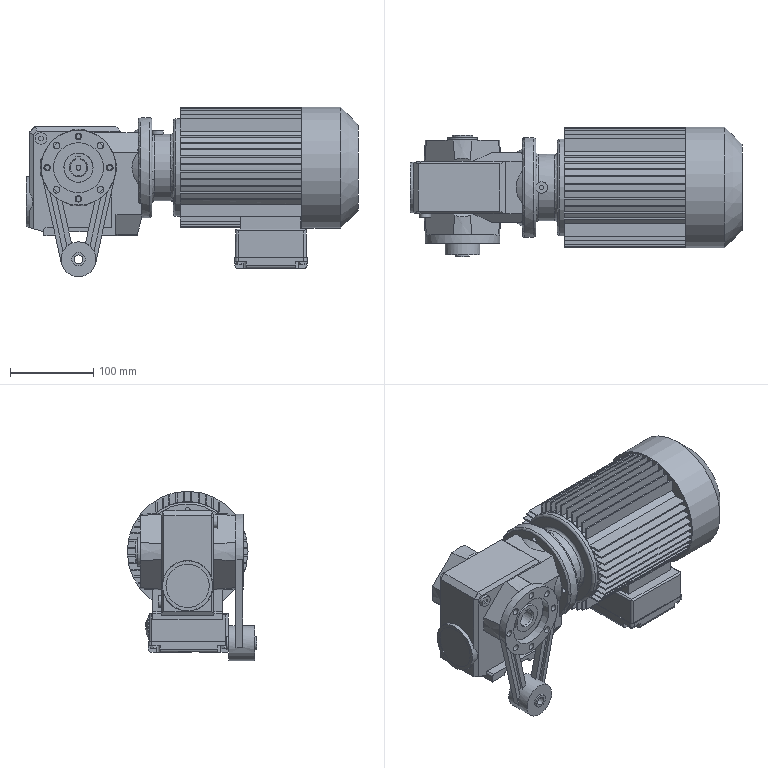Part | STEP file | SA37TDT80N4 | 1 solid | 589 faces | box 398.5 x 155.5 x 203.5 mm | volume 5032005 mm3 | plane 478 | cylinder 87 | cone 17 | torus 5 | sphere 2 | commonest cylinder face diameters 8 x21 6 x17 4 x4 7 x4 14 x3 80 x3